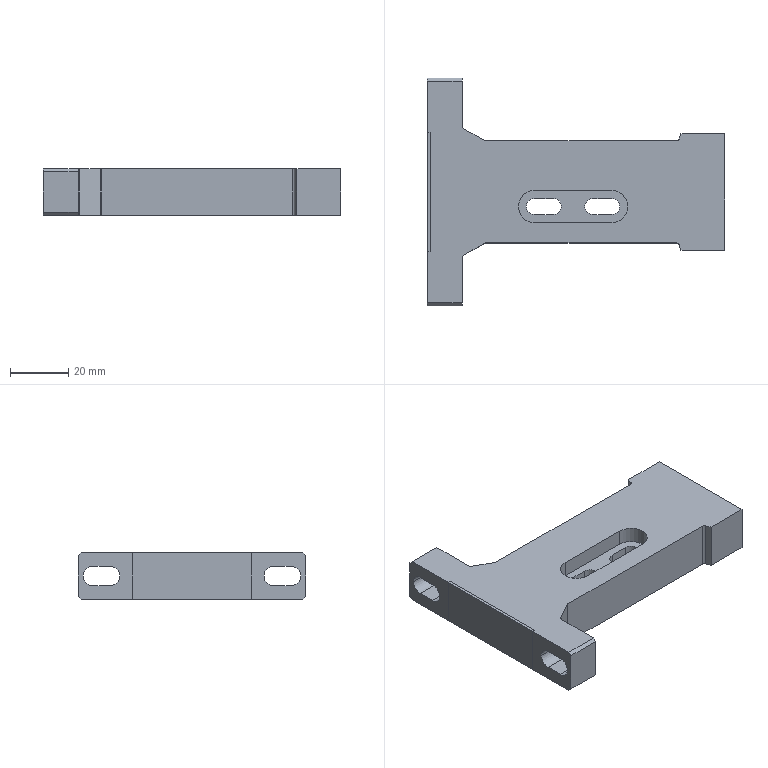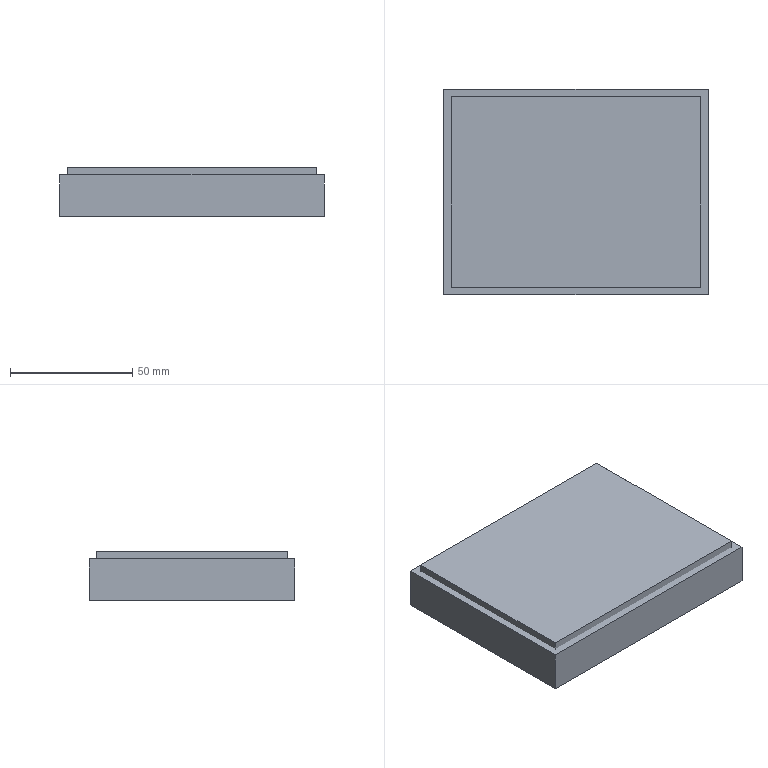CAM job | NX | 3+2 milling, drilling | part box 102 x 78 x 16 mm | stock box 108 x 84 x 20 mm
Tools:
number,name,description,diameter,corner_radius,flute_length,length,flutes
1,D63,Milling Tool-5 Parameters,63.0,0.0,50.0,75.0,2
10,D10,Milling Tool-5 Parameters,10.0,0.0,50.0,75.0,2
11,D10JING,Milling Tool-5 Parameters,10.0,0.0,50.0,75.0,2
7,D6A45,Milling Tool-5 Parameters,6.0,0.0,3.0,3.0,2
4,D4,Milling Tool-5 Parameters,4.0,0.0,50.0,75.0,2
2,D2,Milling Tool-5 Parameters,2.0,0.0,50.0,75.0,2
6,D6,Milling Tool-5 Parameters,6.0,0.0,50.0,75.0,2
14,5.0ZT,Drilling Tool,4.2,0.0,35.0,50.0,2
15,M6,Milling Tool-5 Parameters,4.2,0.0,30.0,30.0,4
13,3.8ZT,Drilling Tool,3.8,0.0,35.0,50.0,2
12,4.0JD,Milling Tool-5 Parameters,4.0,0.0,30.0,30.0,4
Operations:
program,operation,operation_type,tool,method,geometry_group,spindle_rpm,surface_speed,feed_per_tooth,feed_cut,feed_plunge,cut_length_mm,path_length_mm,cut_time_min,machine_time_min
1,FLOOR_WALL,VolumeBased25DMillingOperation,D63,METHOD,A,6500.0,1286.0,0.0962,1250.0,100.0,583.797,637.797,0.467,0.4724
1,ADAPTIVE_MILLING,CavityMilling,D10,METHOD,A,9500.0,298.0,0.1579,3000.0,1000.0,11648.826,11943.531,3.884,3.914
1,ZLEVEL_PROFILE_COPY_COPY_1,ZLevelMilling,D10JING,METHOD,A,9500.0,298.0,0.0632,1200.0,100.0,398.462,484.462,0.3321,0.3407
1,ZLEVEL_PROFILE_COPY_COPY_1_COPY_1,ZLevelMilling,D6,METHOD,A,9500.0,179.0,0.1158,2200.0,100.0,820.784,884.184,0.3731,0.3794
1,ZLEVEL_PROFILE_COPY_COPY_1_COPY_2,ZLevelMilling,D6,METHOD,A,9500.0,298.0,0.0632,1200.0,100.0,76.577,141.577,0.0638,0.0703
1,ZLEVEL_PROFILE_COPY_COPY_1_COPY,ZLevelMilling,D4,METHOD,A,9500.0,119.0,0.0737,1400.0,100.0,1415.421,2868.364,1.011,1.156
1,ZLEVEL_PROFILE_COPY_COPY_1_COPY_1_COPY,ZLevelMilling,D4,METHOD,A,9500.0,119.0,0.0737,1400.0,100.0,1052.976,1227.535,0.7521,0.7696
1,ZLEVEL_PROFILE_COPY_COPY_1_COPY_COPY,ZLevelMilling,D2,METHOD,A,9500.0,59.0,0.0526,1000.0,100.0,2648.716,4400.847,2.649,2.824
1,ZLEVEL_PROFILE_1_COPY_1,ZLevelMilling,D6A45,METHOD,A,9500.0,179.0,0.0526,1000.0,100.0,455.375,628.261,0.4554,0.4727
2,FLOOR_WALL_COPY,VolumeBased25DMillingOperation,D63,METHOD,B,6500.0,1286.0,0.0962,1250.0,100.0,2239.188,2979.084,1.791,1.865
2,FLOOR_WALL_COPY_1,VolumeBased25DMillingOperation,D63,METHOD,B,6500.0,1286.0,0.0962,1250.0,100.0,559.797,613.797,0.4478,0.4532
2,ZLEVEL_PROFILE_COPY_COPY_1_COPY_3,ZLevelMilling,D10JING,METHOD,B,9500.0,298.0,0.0632,1200.0,100.0,702.863,837.366,0.5857,0.5992
2,ZLEVEL_PROFILE_1_COPY_1_COPY,ZLevelMilling,D6A45,METHOD,B,9500.0,179.0,0.0526,1000.0,100.0,552.329,776.059,0.5523,0.5747
2,ZLEVEL_PROFILE_1_COPY_1_COPY_COPY,ZLevelMilling,D6A45,METHOD,B,9500.0,179.0,0.0526,1000.0,100.0,87.617,543.143,0.0876,0.1332
3,ZLEVEL_PROFILE_COPY_COPY_1_COPY_1_COPY_COPY,ZLevelMilling,D4,METHOD,C,9500.0,119.0,0.0737,1400.0,100.0,1714.258,1922.108,1.224,1.245
3,FLOOR_WALL_1,VolumeBased25DMillingOperation,D10JING,METHOD,C,9500.0,0.0,0.0,1250.0,100.0,273.78,512.785,0.219,0.2429
3,ZLEVEL_PROFILE_1_COPY_1_COPY_COPY_1,ZLevelMilling,D6A45,METHOD,C,9500.0,179.0,0.0526,1000.0,100.0,261.741,526.719,0.2617,0.2882
4,DRILLING_COPY_1,Operation,D6A45,METHOD,D,5000.0,94.0,0.025,250.0,0.0,11.2,110.579,0.0448,0.0547
4,DRILLING_COPY_1_COPY,Operation,D6A45,METHOD,D,5000.0,94.0,0.025,250.0,0.0,10.2,91.944,0.0408,0.049
4,DRILLING_COPY,Operation,5.0ZT,METHOD,D,2000.0,39.0,0.0375,150.0,0.0,38.524,165.227,0.2568,0.2695
4,DRILLING_COPY_COPY,Operation,M6,METHOD,D,200.0,2.0,0.0013,1.0,0.0,36.0,160.179,36.0,36.012
4,DRILLING_COPY_COPY_1,Operation,3.8ZT,METHOD,D,2000.0,39.0,0.0375,150.0,0.0,35.083,141.71,0.2339,0.2446
4,DRILLING_COPY_COPY_1_COPY,Operation,4.0JD,METHOD,D,1000.0,12.0,0.0125,50.0,0.0,32.8,137.144,0.656,0.6664